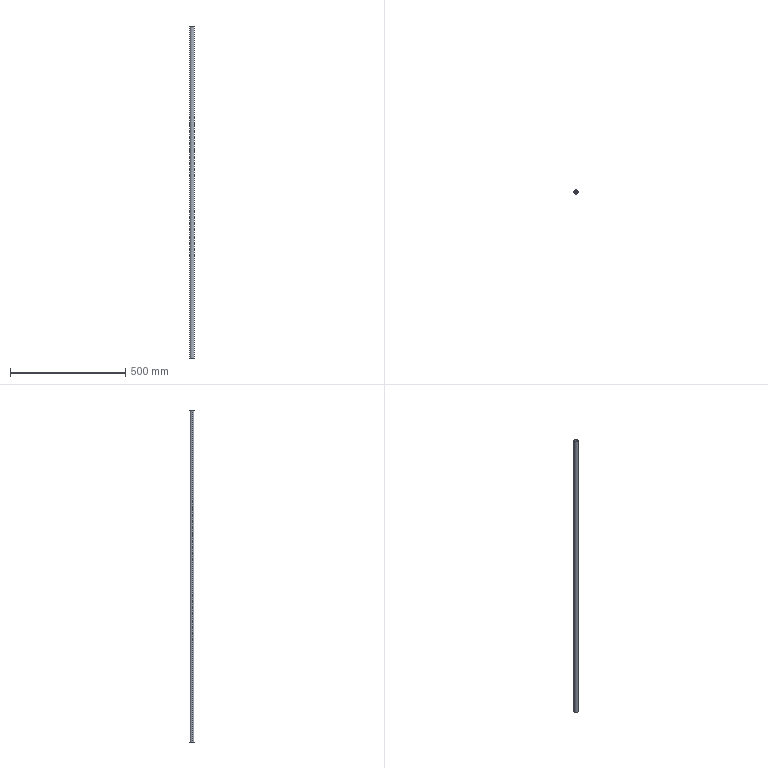Part | STEP file | 1 solid | 6 faces | box 18 x 18 x 1440 mm | volume 175301 mm3 | cylinder 4 | plane 2 | commonest cylinder face diameters 13 x2 18 x2
STEP:
#1=CARTESIAN_POINT('',(0.,0.,0.));
#2=DIRECTION('',(0.,0.,1.));
#3=DIRECTION('',(1.,0.,0.));
#4=AXIS2_PLACEMENT_3D('',#1,#2,#3);
#5=CARTESIAN_POINT('',(-6.5,0.,0.));
#6=VERTEX_POINT('',#5);
#7=CARTESIAN_POINT('',(6.5,0.,0.));
#8=VERTEX_POINT('',#7);
#9=CARTESIAN_POINT('',(0.,0.,0.));
#10=DIRECTION('',(0.,0.,-1.));
#11=DIRECTION('',(-1.,0.,0.));
#12=AXIS2_PLACEMENT_3D('',#9,#10,#11);
#13=CIRCLE('',#12,6.5);
#14=CARTESIAN_POINT('',(0.,0.,1440.));
#15=DIRECTION('',(0.,0.,-1.));
#16=DIRECTION('',(-1.,0.,0.));
#17=AXIS2_PLACEMENT_3D('',#14,#15,#16);
#18=CYLINDRICAL_SURFACE('',#17,6.5);
#19=CARTESIAN_POINT('',(0.,1440.));
#20=DIRECTION('',(1.,0.));
#21=VECTOR('',#20,1.);
#22=LINE('',#19,#21);
#23=(GEOMETRIC_REPRESENTATION_CONTEXT(2)PARAMETRIC_REPRESENTATION_CONTEXT()REPRESENTATION_CONTEXT('',''));
#24=DEFINITIONAL_REPRESENTATION('',(#22),#23);
#25=PCURVE('',#18,#24);
#26=CARTESIAN_POINT('',(0.,0.,0.));
#27=DIRECTION('',(0.,0.,1.));
#28=DIRECTION('',(1.,0.,0.));
#29=AXIS2_PLACEMENT_3D('',#26,#27,#28);
#30=PLANE('',#29);
#31=CARTESIAN_POINT('',(-6.5,0.));
#32=CARTESIAN_POINT('',(-6.5,11.258));
#33=CARTESIAN_POINT('',(3.25,5.629));
#34=CARTESIAN_POINT('',(13.,0.));
#35=CARTESIAN_POINT('',(3.25,-5.629));
#36=CARTESIAN_POINT('',(-6.5,-11.258));
#37=CARTESIAN_POINT('',(-6.5,0.));
#38=(BOUNDED_CURVE()B_SPLINE_CURVE(2,(#31,#32,#33,#34,#35,#36,#37),.UNSPECIFIED.,.T.,.F.)B_SPLINE_CURVE_WITH_KNOTS((1,2,2,2,2,1),(-2.094,0.,2.094,4.189,6.283,8.378),.UNSPECIFIED.)CURVE()GEOMETRIC_REPRESENTATION_ITEM()RATIONAL_B_SPLINE_CURVE((1.,0.5,1.,0.5,1.,0.5,1.))REPRESENTATION_ITEM(''));
#39=(GEOMETRIC_REPRESENTATION_CONTEXT(2)PARAMETRIC_REPRESENTATION_CONTEXT()REPRESENTATION_CONTEXT('',''));
#40=DEFINITIONAL_REPRESENTATION('',(#38),#39);
#41=PCURVE('',#30,#40);
#42=SURFACE_CURVE('',#13,(#25,#41),.PCURVE_S1.);
#43=EDGE_CURVE('',#6,#8,#42,.T.);
#44=ORIENTED_EDGE('',*,*,#43,.F.);
#45=CARTESIAN_POINT('',(-6.5,0.,1440.));
#46=VERTEX_POINT('',#45);
#47=CARTESIAN_POINT('',(-6.5,0.,1440.));
#48=DIRECTION('',(0.,0.,-1.));
#49=VECTOR('',#48,1.);
#50=LINE('',#47,#49);
#51=CARTESIAN_POINT('',(0.,0.));
#52=DIRECTION('',(0.,1.));
#53=VECTOR('',#52,1.);
#54=LINE('',#51,#53);
#55=(GEOMETRIC_REPRESENTATION_CONTEXT(2)PARAMETRIC_REPRESENTATION_CONTEXT()REPRESENTATION_CONTEXT('',''));
#56=DEFINITIONAL_REPRESENTATION('',(#54),#55);
#57=PCURVE('',#18,#56);
#58=CARTESIAN_POINT('',(0.,0.,1440.));
#59=DIRECTION('',(0.,0.,-1.));
#60=DIRECTION('',(-1.,0.,0.));
#61=AXIS2_PLACEMENT_3D('',#58,#59,#60);
#62=CYLINDRICAL_SURFACE('',#61,6.5);
#63=CARTESIAN_POINT('',(6.283,0.));
#64=DIRECTION('',(0.,1.));
#65=VECTOR('',#64,1.);
#66=LINE('',#63,#65);
#67=(GEOMETRIC_REPRESENTATION_CONTEXT(2)PARAMETRIC_REPRESENTATION_CONTEXT()REPRESENTATION_CONTEXT('',''));
#68=DEFINITIONAL_REPRESENTATION('',(#66),#67);
#69=PCURVE('',#62,#68);
#70=SURFACE_CURVE('',#50,(#57,#69),.PCURVE_S1.);
#71=EDGE_CURVE('',#46,#6,#70,.T.);
#72=ORIENTED_EDGE('',*,*,#71,.F.);
#73=CARTESIAN_POINT('',(6.5,0.,1440.));
#74=VERTEX_POINT('',#73);
#75=CARTESIAN_POINT('',(0.,0.,1440.));
#76=DIRECTION('',(0.,0.,-1.));
#77=DIRECTION('',(-1.,0.,0.));
#78=AXIS2_PLACEMENT_3D('',#75,#76,#77);
#79=CIRCLE('',#78,6.5);
#80=CARTESIAN_POINT('',(0.,0.));
#81=DIRECTION('',(1.,0.));
#82=VECTOR('',#81,1.);
#83=LINE('',#80,#82);
#84=(GEOMETRIC_REPRESENTATION_CONTEXT(2)PARAMETRIC_REPRESENTATION_CONTEXT()REPRESENTATION_CONTEXT('',''));
#85=DEFINITIONAL_REPRESENTATION('',(#83),#84);
#86=PCURVE('',#18,#85);
#87=CARTESIAN_POINT('',(0.,0.,1440.));
#88=DIRECTION('',(0.,0.,1.));
#89=DIRECTION('',(1.,0.,0.));
#90=AXIS2_PLACEMENT_3D('',#87,#88,#89);
#91=PLANE('',#90);
#92=CARTESIAN_POINT('',(-6.5,0.));
#93=CARTESIAN_POINT('',(-6.5,11.258));
#94=CARTESIAN_POINT('',(3.25,5.629));
#95=CARTESIAN_POINT('',(13.,0.));
#96=CARTESIAN_POINT('',(3.25,-5.629));
#97=CARTESIAN_POINT('',(-6.5,-11.258));
#98=CARTESIAN_POINT('',(-6.5,0.));
#99=(BOUNDED_CURVE()B_SPLINE_CURVE(2,(#92,#93,#94,#95,#96,#97,#98),.UNSPECIFIED.,.T.,.F.)B_SPLINE_CURVE_WITH_KNOTS((1,2,2,2,2,1),(-2.094,0.,2.094,4.189,6.283,8.378),.UNSPECIFIED.)CURVE()GEOMETRIC_REPRESENTATION_ITEM()RATIONAL_B_SPLINE_CURVE((1.,0.5,1.,0.5,1.,0.5,1.))REPRESENTATION_ITEM(''));
#100=(GEOMETRIC_REPRESENTATION_CONTEXT(2)PARAMETRIC_REPRESENTATION_CONTEXT()REPRESENTATION_CONTEXT('',''));
#101=DEFINITIONAL_REPRESENTATION('',(#99),#100);
#102=PCURVE('',#91,#101);
#103=SURFACE_CURVE('',#79,(#86,#102),.PCURVE_S1.);
#104=EDGE_CURVE('',#46,#74,#103,.T.);
#105=ORIENTED_EDGE('',*,*,#104,.T.);
#106=CARTESIAN_POINT('',(6.5,0.,1440.));
#107=DIRECTION('',(0.,0.,-1.));
#108=VECTOR('',#107,1.);
#109=LINE('',#106,#108);
#110=CARTESIAN_POINT('',(3.142,0.));
#111=DIRECTION('',(0.,1.));
#112=VECTOR('',#111,1.);
#113=LINE('',#110,#112);
#114=(GEOMETRIC_REPRESENTATION_CONTEXT(2)PARAMETRIC_REPRESENTATION_CONTEXT()REPRESENTATION_CONTEXT('',''));
#115=DEFINITIONAL_REPRESENTATION('',(#113),#114);
#116=PCURVE('',#18,#115);
#117=CARTESIAN_POINT('',(3.142,0.));
#118=DIRECTION('',(0.,1.));
#119=VECTOR('',#118,1.);
#120=LINE('',#117,#119);
#121=(GEOMETRIC_REPRESENTATION_CONTEXT(2)PARAMETRIC_REPRESENTATION_CONTEXT()REPRESENTATION_CONTEXT('',''));
#122=DEFINITIONAL_REPRESENTATION('',(#120),#121);
#123=PCURVE('',#62,#122);
#124=SURFACE_CURVE('',#109,(#116,#123),.PCURVE_S1.);
#125=EDGE_CURVE('',#74,#8,#124,.T.);
#126=ORIENTED_EDGE('',*,*,#125,.T.);
#127=EDGE_LOOP('',(#44,#72,#105,#126));
#128=FACE_BOUND('',#127,.F.);
#129=ADVANCED_FACE('',(#128),#18,.F.);
#130=ORIENTED_EDGE('',*,*,#104,.T.);
#131=CARTESIAN_POINT('',(0.,0.,1440.));
#132=DIRECTION('',(0.,0.,-1.));
#133=DIRECTION('',(-1.,0.,0.));
#134=AXIS2_PLACEMENT_3D('',#131,#132,#133);
#135=CIRCLE('',#134,6.5);
#136=CARTESIAN_POINT('',(-6.5,0.));
#137=CARTESIAN_POINT('',(-6.5,11.258));
#138=CARTESIAN_POINT('',(3.25,5.629));
#139=CARTESIAN_POINT('',(13.,0.));
#140=CARTESIAN_POINT('',(3.25,-5.629));
#141=CARTESIAN_POINT('',(-6.5,-11.258));
#142=CARTESIAN_POINT('',(-6.5,0.));
#143=(BOUNDED_CURVE()B_SPLINE_CURVE(2,(#136,#137,#138,#139,#140,#141,#142),.UNSPECIFIED.,.T.,.F.)B_SPLINE_CURVE_WITH_KNOTS((1,2,2,2,2,1),(-2.094,0.,2.094,4.189,6.283,8.378),.UNSPECIFIED.)CURVE()GEOMETRIC_REPRESENTATION_ITEM()RATIONAL_B_SPLINE_CURVE((1.,0.5,1.,0.5,1.,0.5,1.))REPRESENTATION_ITEM(''));
#144=(GEOMETRIC_REPRESENTATION_CONTEXT(2)PARAMETRIC_REPRESENTATION_CONTEXT()REPRESENTATION_CONTEXT('',''));
#145=DEFINITIONAL_REPRESENTATION('',(#143),#144);
#146=PCURVE('',#91,#145);
#147=CARTESIAN_POINT('',(0.,0.));
#148=DIRECTION('',(1.,0.));
#149=VECTOR('',#148,1.);
#150=LINE('',#147,#149);
#151=(GEOMETRIC_REPRESENTATION_CONTEXT(2)PARAMETRIC_REPRESENTATION_CONTEXT()REPRESENTATION_CONTEXT('',''));
#152=DEFINITIONAL_REPRESENTATION('',(#150),#151);
#153=PCURVE('',#62,#152);
#154=SURFACE_CURVE('',#135,(#146,#153),.PCURVE_S1.);
#155=EDGE_CURVE('',#74,#46,#154,.T.);
#156=ORIENTED_EDGE('',*,*,#155,.T.);
#157=EDGE_LOOP('',(#130,#156));
#158=FACE_BOUND('',#157,.T.);
#159=CARTESIAN_POINT('',(-9.,0.,1440.));
#160=VERTEX_POINT('',#159);
#161=CARTESIAN_POINT('',(9.,0.,1440.));
#162=VERTEX_POINT('',#161);
#163=CARTESIAN_POINT('',(0.,0.,1440.));
#164=DIRECTION('',(0.,0.,-1.));
#165=DIRECTION('',(-1.,0.,0.));
#166=AXIS2_PLACEMENT_3D('',#163,#164,#165);
#167=CIRCLE('',#166,9.);
#168=CARTESIAN_POINT('',(-9.,0.));
#169=CARTESIAN_POINT('',(-9.,15.588));
#170=CARTESIAN_POINT('',(4.5,7.794));
#171=CARTESIAN_POINT('',(18.,0.));
#172=CARTESIAN_POINT('',(4.5,-7.794));
#173=CARTESIAN_POINT('',(-9.,-15.588));
#174=CARTESIAN_POINT('',(-9.,0.));
#175=(BOUNDED_CURVE()B_SPLINE_CURVE(2,(#168,#169,#170,#171,#172,#173,#174),.UNSPECIFIED.,.T.,.F.)B_SPLINE_CURVE_WITH_KNOTS((1,2,2,2,2,1),(-2.094,0.,2.094,4.189,6.283,8.378),.UNSPECIFIED.)CURVE()GEOMETRIC_REPRESENTATION_ITEM()RATIONAL_B_SPLINE_CURVE((1.,0.5,1.,0.5,1.,0.5,1.))REPRESENTATION_ITEM(''));
#176=(GEOMETRIC_REPRESENTATION_CONTEXT(2)PARAMETRIC_REPRESENTATION_CONTEXT()REPRESENTATION_CONTEXT('',''));
#177=DEFINITIONAL_REPRESENTATION('',(#175),#176);
#178=PCURVE('',#91,#177);
#179=CARTESIAN_POINT('',(0.,0.,1440.));
#180=DIRECTION('',(0.,0.,-1.));
#181=DIRECTION('',(-1.,0.,0.));
#182=AXIS2_PLACEMENT_3D('',#179,#180,#181);
#183=CYLINDRICAL_SURFACE('',#182,9.);
#184=CARTESIAN_POINT('',(0.,0.));
#185=DIRECTION('',(1.,0.));
#186=VECTOR('',#185,1.);
#187=LINE('',#184,#186);
#188=(GEOMETRIC_REPRESENTATION_CONTEXT(2)PARAMETRIC_REPRESENTATION_CONTEXT()REPRESENTATION_CONTEXT('',''));
#189=DEFINITIONAL_REPRESENTATION('',(#187),#188);
#190=PCURVE('',#183,#189);
#191=SURFACE_CURVE('',#167,(#178,#190),.PCURVE_S1.);
#192=EDGE_CURVE('',#160,#162,#191,.T.);
#193=ORIENTED_EDGE('',*,*,#192,.F.);
#194=CARTESIAN_POINT('',(0.,0.,1440.));
#195=DIRECTION('',(0.,0.,-1.));
#196=DIRECTION('',(-1.,0.,0.));
#197=AXIS2_PLACEMENT_3D('',#194,#195,#196);
#198=CIRCLE('',#197,9.);
#199=CARTESIAN_POINT('',(-9.,0.));
#200=CARTESIAN_POINT('',(-9.,15.588));
#201=CARTESIAN_POINT('',(4.5,7.794));
#202=CARTESIAN_POINT('',(18.,0.));
#203=CARTESIAN_POINT('',(4.5,-7.794));
#204=CARTESIAN_POINT('',(-9.,-15.588));
#205=CARTESIAN_POINT('',(-9.,0.));
#206=(BOUNDED_CURVE()B_SPLINE_CURVE(2,(#199,#200,#201,#202,#203,#204,#205),.UNSPECIFIED.,.T.,.F.)B_SPLINE_CURVE_WITH_KNOTS((1,2,2,2,2,1),(-2.094,0.,2.094,4.189,6.283,8.378),.UNSPECIFIED.)CURVE()GEOMETRIC_REPRESENTATION_ITEM()RATIONAL_B_SPLINE_CURVE((1.,0.5,1.,0.5,1.,0.5,1.))REPRESENTATION_ITEM(''));
#207=(GEOMETRIC_REPRESENTATION_CONTEXT(2)PARAMETRIC_REPRESENTATION_CONTEXT()REPRESENTATION_CONTEXT('',''));
#208=DEFINITIONAL_REPRESENTATION('',(#206),#207);
#209=PCURVE('',#91,#208);
#210=CARTESIAN_POINT('',(0.,0.,1440.));
#211=DIRECTION('',(0.,0.,-1.));
#212=DIRECTION('',(-1.,0.,0.));
#213=AXIS2_PLACEMENT_3D('',#210,#211,#212);
#214=CYLINDRICAL_SURFACE('',#213,9.);
#215=CARTESIAN_POINT('',(0.,0.));
#216=DIRECTION('',(1.,0.));
#217=VECTOR('',#216,1.);
#218=LINE('',#215,#217);
#219=(GEOMETRIC_REPRESENTATION_CONTEXT(2)PARAMETRIC_REPRESENTATION_CONTEXT()REPRESENTATION_CONTEXT('',''));
#220=DEFINITIONAL_REPRESENTATION('',(#218),#219);
#221=PCURVE('',#214,#220);
#222=SURFACE_CURVE('',#198,(#209,#221),.PCURVE_S1.);
#223=EDGE_CURVE('',#162,#160,#222,.T.);
#224=ORIENTED_EDGE('',*,*,#223,.F.);
#225=EDGE_LOOP('',(#193,#224));
#226=FACE_BOUND('',#225,.T.);
#227=ADVANCED_FACE('',(#158,#226),#91,.T.);
#228=ORIENTED_EDGE('',*,*,#43,.F.);
#229=CARTESIAN_POINT('',(0.,0.,0.));
#230=DIRECTION('',(0.,0.,-1.));
#231=DIRECTION('',(-1.,0.,0.));
#232=AXIS2_PLACEMENT_3D('',#229,#230,#231);
#233=CIRCLE('',#232,6.5);
#234=CARTESIAN_POINT('',(-6.5,0.));
#235=CARTESIAN_POINT('',(-6.5,11.258));
#236=CARTESIAN_POINT('',(3.25,5.629));
#237=CARTESIAN_POINT('',(13.,0.));
#238=CARTESIAN_POINT('',(3.25,-5.629));
#239=CARTESIAN_POINT('',(-6.5,-11.258));
#240=CARTESIAN_POINT('',(-6.5,0.));
#241=(BOUNDED_CURVE()B_SPLINE_CURVE(2,(#234,#235,#236,#237,#238,#239,#240),.UNSPECIFIED.,.T.,.F.)B_SPLINE_CURVE_WITH_KNOTS((1,2,2,2,2,1),(-2.094,0.,2.094,4.189,6.283,8.378),.UNSPECIFIED.)CURVE()GEOMETRIC_REPRESENTATION_ITEM()RATIONAL_B_SPLINE_CURVE((1.,0.5,1.,0.5,1.,0.5,1.))REPRESENTATION_ITEM(''));
#242=(GEOMETRIC_REPRESENTATION_CONTEXT(2)PARAMETRIC_REPRESENTATION_CONTEXT()REPRESENTATION_CONTEXT('',''));
#243=DEFINITIONAL_REPRESENTATION('',(#241),#242);
#244=PCURVE('',#30,#243);
#245=CARTESIAN_POINT('',(0.,1440.));
#246=DIRECTION('',(1.,0.));
#247=VECTOR('',#246,1.);
#248=LINE('',#245,#247);
#249=(GEOMETRIC_REPRESENTATION_CONTEXT(2)PARAMETRIC_REPRESENTATION_CONTEXT()REPRESENTATION_CONTEXT('',''));
#250=DEFINITIONAL_REPRESENTATION('',(#248),#249);
#251=PCURVE('',#62,#250);
#252=SURFACE_CURVE('',#233,(#244,#251),.PCURVE_S1.);
#253=EDGE_CURVE('',#8,#6,#252,.T.);
#254=ORIENTED_EDGE('',*,*,#253,.F.);
#255=EDGE_LOOP('',(#228,#254));
#256=FACE_BOUND('',#255,.T.);
#257=CARTESIAN_POINT('',(-9.,0.,0.));
#258=VERTEX_POINT('',#257);
#259=CARTESIAN_POINT('',(9.,0.,0.));
#260=VERTEX_POINT('',#259);
#261=CARTESIAN_POINT('',(0.,0.,0.));
#262=DIRECTION('',(0.,0.,1.));
#263=DIRECTION('',(-1.,0.,0.));
#264=AXIS2_PLACEMENT_3D('',#261,#262,#263);
#265=CIRCLE('',#264,9.);
#266=CARTESIAN_POINT('',(0.,0.));
#267=DIRECTION('',(-1.,0.));
#268=AXIS2_PLACEMENT_2D('',#266,#267);
#269=CIRCLE('',#268,9.);
#270=(GEOMETRIC_REPRESENTATION_CONTEXT(2)PARAMETRIC_REPRESENTATION_CONTEXT()REPRESENTATION_CONTEXT('',''));
#271=DEFINITIONAL_REPRESENTATION('',(#269),#270);
#272=PCURVE('',#30,#271);
#273=CARTESIAN_POINT('',(6.283,1440.));
#274=DIRECTION('',(-1.,0.));
#275=VECTOR('',#274,1.);
#276=LINE('',#273,#275);
#277=(GEOMETRIC_REPRESENTATION_CONTEXT(2)PARAMETRIC_REPRESENTATION_CONTEXT()REPRESENTATION_CONTEXT('',''));
#278=DEFINITIONAL_REPRESENTATION('',(#276),#277);
#279=PCURVE('',#214,#278);
#280=SURFACE_CURVE('',#265,(#272,#279),.PCURVE_S1.);
#281=EDGE_CURVE('',#258,#260,#280,.T.);
#282=ORIENTED_EDGE('',*,*,#281,.F.);
#283=CARTESIAN_POINT('',(0.,0.,0.));
#284=DIRECTION('',(0.,0.,1.));
#285=DIRECTION('',(-1.,0.,0.));
#286=AXIS2_PLACEMENT_3D('',#283,#284,#285);
#287=CIRCLE('',#286,9.);
#288=CARTESIAN_POINT('',(0.,0.));
#289=DIRECTION('',(-1.,0.));
#290=AXIS2_PLACEMENT_2D('',#288,#289);
#291=CIRCLE('',#290,9.);
#292=(GEOMETRIC_REPRESENTATION_CONTEXT(2)PARAMETRIC_REPRESENTATION_CONTEXT()REPRESENTATION_CONTEXT('',''));
#293=DEFINITIONAL_REPRESENTATION('',(#291),#292);
#294=PCURVE('',#30,#293);
#295=CARTESIAN_POINT('',(6.283,1440.));
#296=DIRECTION('',(-1.,0.));
#297=VECTOR('',#296,1.);
#298=LINE('',#295,#297);
#299=(GEOMETRIC_REPRESENTATION_CONTEXT(2)PARAMETRIC_REPRESENTATION_CONTEXT()REPRESENTATION_CONTEXT('',''));
#300=DEFINITIONAL_REPRESENTATION('',(#298),#299);
#301=PCURVE('',#183,#300);
#302=SURFACE_CURVE('',#287,(#294,#301),.PCURVE_S1.);
#303=EDGE_CURVE('',#260,#258,#302,.T.);
#304=ORIENTED_EDGE('',*,*,#303,.F.);
#305=EDGE_LOOP('',(#282,#304));
#306=FACE_BOUND('',#305,.T.);
#307=ADVANCED_FACE('',(#256,#306),#30,.F.);
#308=CARTESIAN_POINT('',(9.,0.,1440.));
#309=DIRECTION('',(0.,0.,-1.));
#310=VECTOR('',#309,1.);
#311=LINE('',#308,#310);
#312=CARTESIAN_POINT('',(3.142,0.));
#313=DIRECTION('',(0.,1.));
#314=VECTOR('',#313,1.);
#315=LINE('',#312,#314);
#316=(GEOMETRIC_REPRESENTATION_CONTEXT(2)PARAMETRIC_REPRESENTATION_CONTEXT()REPRESENTATION_CONTEXT('',''));
#317=DEFINITIONAL_REPRESENTATION('',(#315),#316);
#318=PCURVE('',#214,#317);
#319=CARTESIAN_POINT('',(3.142,0.));
#320=DIRECTION('',(0.,1.));
#321=VECTOR('',#320,1.);
#322=LINE('',#319,#321);
#323=(GEOMETRIC_REPRESENTATION_CONTEXT(2)PARAMETRIC_REPRESENTATION_CONTEXT()REPRESENTATION_CONTEXT('',''));
#324=DEFINITIONAL_REPRESENTATION('',(#322),#323);
#325=PCURVE('',#183,#324);
#326=SURFACE_CURVE('',#311,(#318,#325),.PCURVE_S1.);
#327=EDGE_CURVE('',#162,#260,#326,.T.);
#328=ORIENTED_EDGE('',*,*,#327,.F.);
#329=ORIENTED_EDGE('',*,*,#223,.T.);
#330=CARTESIAN_POINT('',(-9.,0.,1440.));
#331=DIRECTION('',(0.,0.,-1.));
#332=VECTOR('',#331,1.);
#333=LINE('',#330,#332);
#334=CARTESIAN_POINT('',(6.283,0.));
#335=DIRECTION('',(0.,1.));
#336=VECTOR('',#335,1.);
#337=LINE('',#334,#336);
#338=(GEOMETRIC_REPRESENTATION_CONTEXT(2)PARAMETRIC_REPRESENTATION_CONTEXT()REPRESENTATION_CONTEXT('',''));
#339=DEFINITIONAL_REPRESENTATION('',(#337),#338);
#340=PCURVE('',#214,#339);
#341=CARTESIAN_POINT('',(0.,0.));
#342=DIRECTION('',(0.,1.));
#343=VECTOR('',#342,1.);
#344=LINE('',#341,#343);
#345=(GEOMETRIC_REPRESENTATION_CONTEXT(2)PARAMETRIC_REPRESENTATION_CONTEXT()REPRESENTATION_CONTEXT('',''));
#346=DEFINITIONAL_REPRESENTATION('',(#344),#345);
#347=PCURVE('',#183,#346);
#348=SURFACE_CURVE('',#333,(#340,#347),.PCURVE_S1.);
#349=EDGE_CURVE('',#160,#258,#348,.T.);
#350=ORIENTED_EDGE('',*,*,#349,.T.);
#351=ORIENTED_EDGE('',*,*,#281,.T.);
#352=EDGE_LOOP('',(#328,#329,#350,#351));
#353=FACE_BOUND('',#352,.T.);
#354=ADVANCED_FACE('',(#353),#214,.T.);
#355=ORIENTED_EDGE('',*,*,#71,.T.);
#356=ORIENTED_EDGE('',*,*,#253,.F.);
#357=ORIENTED_EDGE('',*,*,#125,.F.);
#358=ORIENTED_EDGE('',*,*,#155,.T.);
#359=EDGE_LOOP('',(#355,#356,#357,#358));
#360=FACE_BOUND('',#359,.F.);
#361=ADVANCED_FACE('',(#360),#62,.F.);
#362=ORIENTED_EDGE('',*,*,#192,.T.);
#363=ORIENTED_EDGE('',*,*,#327,.T.);
#364=ORIENTED_EDGE('',*,*,#303,.T.);
#365=ORIENTED_EDGE('',*,*,#349,.F.);
#366=EDGE_LOOP('',(#362,#363,#364,#365));
#367=FACE_BOUND('',#366,.T.);
#368=ADVANCED_FACE('',(#367),#183,.T.);
#369=CLOSED_SHELL('',(#129,#227,#307,#354,#361,#368));
#370=MANIFOLD_SOLID_BREP('',#369);
#371=(LENGTH_UNIT()NAMED_UNIT(*)SI_UNIT(.MILLI.,.METRE.));
#372=UNCERTAINTY_MEASURE_WITH_UNIT(LENGTH_MEASURE(0.0000001),#371,'','');
#373=(NAMED_UNIT(*)PLANE_ANGLE_UNIT()SI_UNIT($,.RADIAN.));
#374=(NAMED_UNIT(*)SI_UNIT($,.STERADIAN.)SOLID_ANGLE_UNIT());
#375=(GEOMETRIC_REPRESENTATION_CONTEXT(3)GLOBAL_UNCERTAINTY_ASSIGNED_CONTEXT((#372))GLOBAL_UNIT_ASSIGNED_CONTEXT((#371,#373,#374))REPRESENTATION_CONTEXT('',''));
#376=ADVANCED_BREP_SHAPE_REPRESENTATION('',(#4,#370),#375);